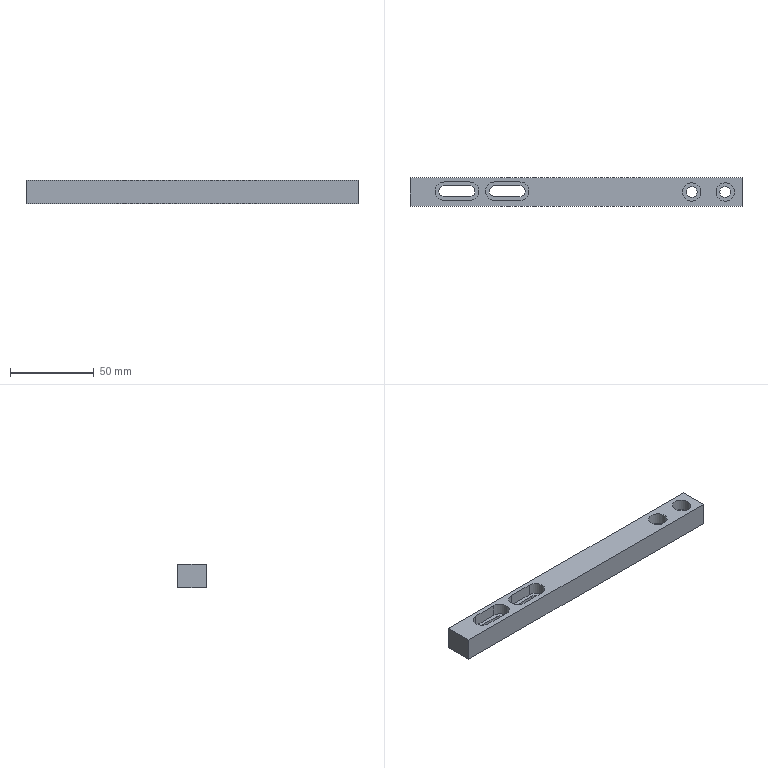Part | STEP file | solid 130 | 1 solid | 39 faces | box 198 x 17 x 14 mm | volume 37768 mm3 | plane 23 | cylinder 16 | commonest cylinder face diameters 6.5 x6 11 x6 8 x4